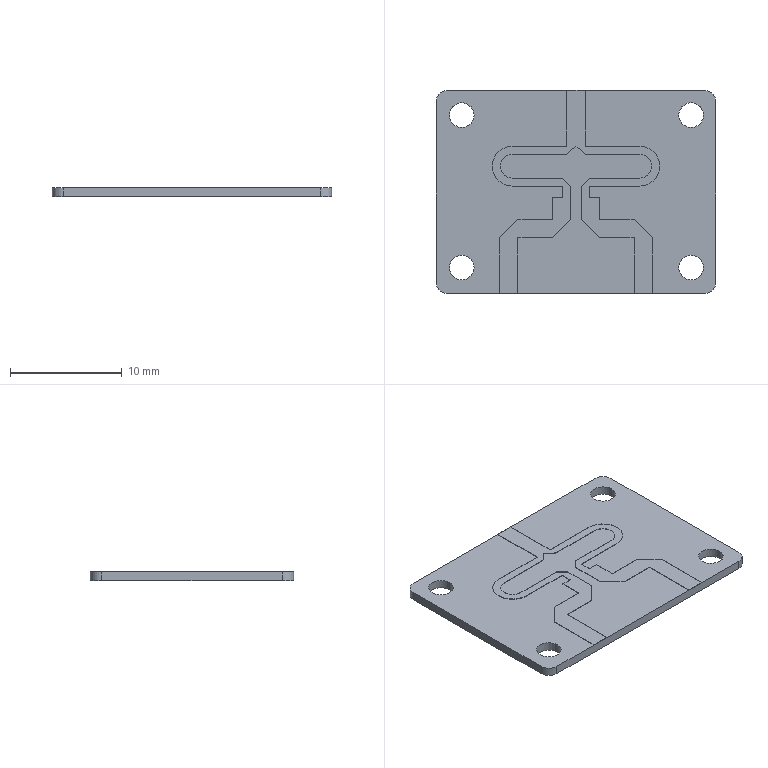Part | STEP file | 1 to 2 power divider PCB | 2 solids | 57 faces | box 25 x 18.18 x 0.832 mm | volume 351.83 mm3 | plane 45 | cylinder 12 | commonest cylinder face diameters 2 x4 2.2 x4 2.12 x2 3.56 x2